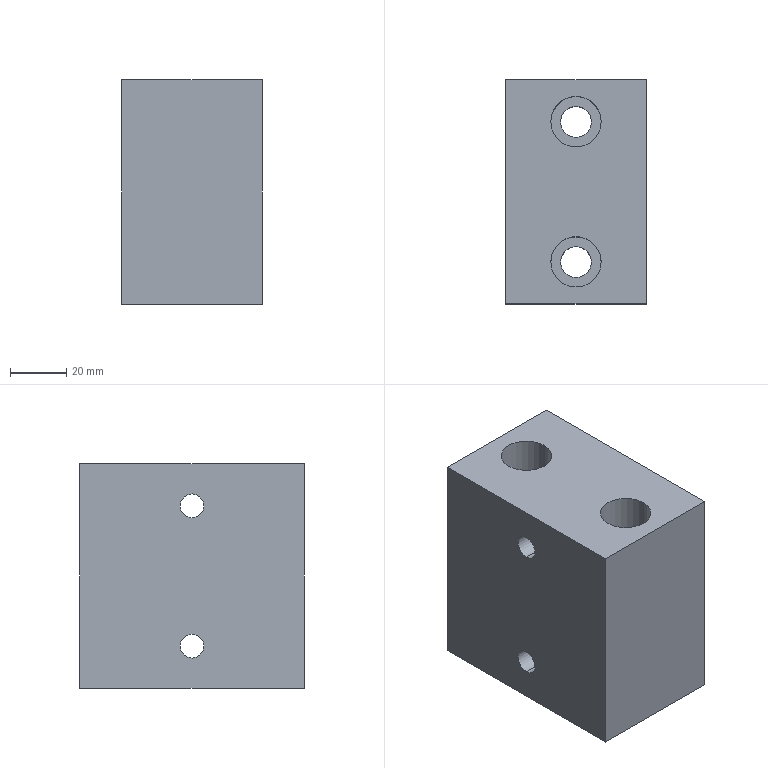Part | SolidWorks | features HoleWzd 2, Extrusion 1 | 1 solid | 20 faces | box 50 x 80 x 80 mm | volume 289554 mm3 | cylinder 12 | plane 8 | commonest cylinder face diameters 8.5 x4 11 x4 18 x4
STEP:
#1=CARTESIAN_POINT('',(0.,0.,-20.75));
#2=VERTEX_POINT('',#1);
#3=CARTESIAN_POINT('',(0.,0.,-29.25));
#4=VERTEX_POINT('',#3);
#5=CARTESIAN_POINT('',(0.,0.,-25.));
#6=DIRECTION('',(1.,0.,0.));
#7=DIRECTION('',(0.,0.,-1.));
#8=AXIS2_PLACEMENT_3D('',#5,#6,#7);
#9=CIRCLE('',#8,4.25);
#10=EDGE_CURVE('',#2,#4,#9,.T.);
#11=ORIENTED_EDGE('',*,*,#10,.F.);
#12=CARTESIAN_POINT('',(50.,0.,-20.75));
#13=VERTEX_POINT('',#12);
#14=CARTESIAN_POINT('',(50.,0.,-20.75));
#15=DIRECTION('',(1.,0.,0.));
#16=VECTOR('',#15,1000.);
#17=LINE('',#14,#16);
#18=EDGE_CURVE('',#2,#13,#17,.T.);
#19=ORIENTED_EDGE('',*,*,#18,.T.);
#20=CARTESIAN_POINT('',(50.,0.,-29.25));
#21=VERTEX_POINT('',#20);
#22=CARTESIAN_POINT('',(50.,0.,-25.));
#23=DIRECTION('',(1.,0.,0.));
#24=DIRECTION('',(0.,0.,-1.));
#25=AXIS2_PLACEMENT_3D('',#22,#23,#24);
#26=CIRCLE('',#25,4.25);
#27=EDGE_CURVE('',#13,#21,#26,.T.);
#28=ORIENTED_EDGE('',*,*,#27,.T.);
#29=CARTESIAN_POINT('',(50.,0.,-29.25));
#30=DIRECTION('',(1.,0.,0.));
#31=VECTOR('',#30,1000.);
#32=LINE('',#29,#31);
#33=EDGE_CURVE('',#4,#21,#32,.T.);
#34=ORIENTED_EDGE('',*,*,#33,.F.);
#35=EDGE_LOOP('',(#11,#19,#28,#34));
#36=FACE_OUTER_BOUND('',#35,.T.);
#37=CARTESIAN_POINT('',(50.,0.,-25.));
#38=DIRECTION('',(1.,0.,0.));
#39=DIRECTION('',(0.,0.,-1.));
#40=AXIS2_PLACEMENT_3D('',#37,#38,#39);
#41=CYLINDRICAL_SURFACE('',#40,4.25);
#42=ADVANCED_FACE('',(#36),#41,.F.);
#43=CARTESIAN_POINT('',(0.,0.,29.25));
#44=VERTEX_POINT('',#43);
#45=CARTESIAN_POINT('',(0.,0.,20.75));
#46=VERTEX_POINT('',#45);
#47=CARTESIAN_POINT('',(0.,0.,25.));
#48=DIRECTION('',(1.,0.,0.));
#49=DIRECTION('',(0.,0.,-1.));
#50=AXIS2_PLACEMENT_3D('',#47,#48,#49);
#51=CIRCLE('',#50,4.25);
#52=EDGE_CURVE('',#44,#46,#51,.T.);
#53=ORIENTED_EDGE('',*,*,#52,.F.);
#54=CARTESIAN_POINT('',(50.,0.,29.25));
#55=VERTEX_POINT('',#54);
#56=CARTESIAN_POINT('',(50.,0.,29.25));
#57=DIRECTION('',(1.,0.,0.));
#58=VECTOR('',#57,1000.);
#59=LINE('',#56,#58);
#60=EDGE_CURVE('',#44,#55,#59,.T.);
#61=ORIENTED_EDGE('',*,*,#60,.T.);
#62=CARTESIAN_POINT('',(50.,0.,20.75));
#63=VERTEX_POINT('',#62);
#64=CARTESIAN_POINT('',(50.,0.,25.));
#65=DIRECTION('',(1.,0.,0.));
#66=DIRECTION('',(0.,0.,-1.));
#67=AXIS2_PLACEMENT_3D('',#64,#65,#66);
#68=CIRCLE('',#67,4.25);
#69=EDGE_CURVE('',#55,#63,#68,.T.);
#70=ORIENTED_EDGE('',*,*,#69,.T.);
#71=CARTESIAN_POINT('',(50.,0.,20.75));
#72=DIRECTION('',(1.,0.,0.));
#73=VECTOR('',#72,1000.);
#74=LINE('',#71,#73);
#75=EDGE_CURVE('',#46,#63,#74,.T.);
#76=ORIENTED_EDGE('',*,*,#75,.F.);
#77=EDGE_LOOP('',(#53,#61,#70,#76));
#78=FACE_OUTER_BOUND('',#77,.T.);
#79=CARTESIAN_POINT('',(50.,0.,25.));
#80=DIRECTION('',(1.,0.,0.));
#81=DIRECTION('',(0.,0.,-1.));
#82=AXIS2_PLACEMENT_3D('',#79,#80,#81);
#83=CYLINDRICAL_SURFACE('',#82,4.25);
#84=ADVANCED_FACE('',(#78),#83,.F.);
#85=CARTESIAN_POINT('',(16.,25.,10.));
#86=VERTEX_POINT('',#85);
#87=CARTESIAN_POINT('',(34.,25.,10.));
#88=VERTEX_POINT('',#87);
#89=CARTESIAN_POINT('',(25.,25.,10.));
#90=DIRECTION('',(0.,0.,1.));
#91=DIRECTION('',(1.,0.,0.));
#92=AXIS2_PLACEMENT_3D('',#89,#90,#91);
#93=CIRCLE('',#92,9.);
#94=EDGE_CURVE('',#86,#88,#93,.T.);
#95=ORIENTED_EDGE('',*,*,#94,.F.);
#96=CARTESIAN_POINT('',(16.,25.,40.));
#97=VERTEX_POINT('',#96);
#98=CARTESIAN_POINT('',(16.,25.,40.));
#99=DIRECTION('',(0.,0.,1.));
#100=VECTOR('',#99,1000.);
#101=LINE('',#98,#100);
#102=EDGE_CURVE('',#86,#97,#101,.T.);
#103=ORIENTED_EDGE('',*,*,#102,.T.);
#104=CARTESIAN_POINT('',(34.,25.,40.));
#105=VERTEX_POINT('',#104);
#106=CARTESIAN_POINT('',(25.,25.,40.));
#107=DIRECTION('',(0.,0.,1.));
#108=DIRECTION('',(1.,0.,0.));
#109=AXIS2_PLACEMENT_3D('',#106,#107,#108);
#110=CIRCLE('',#109,9.);
#111=EDGE_CURVE('',#97,#105,#110,.T.);
#112=ORIENTED_EDGE('',*,*,#111,.T.);
#113=CARTESIAN_POINT('',(34.,25.,40.));
#114=DIRECTION('',(0.,0.,1.));
#115=VECTOR('',#114,1000.);
#116=LINE('',#113,#115);
#117=EDGE_CURVE('',#88,#105,#116,.T.);
#118=ORIENTED_EDGE('',*,*,#117,.F.);
#119=EDGE_LOOP('',(#95,#103,#112,#118));
#120=FACE_OUTER_BOUND('',#119,.T.);
#121=CARTESIAN_POINT('',(25.,25.,40.));
#122=DIRECTION('',(0.,0.,1.));
#123=DIRECTION('',(1.,0.,0.));
#124=AXIS2_PLACEMENT_3D('',#121,#122,#123);
#125=CYLINDRICAL_SURFACE('',#124,9.);
#126=ADVANCED_FACE('',(#120),#125,.F.);
#127=CARTESIAN_POINT('',(19.5,25.,-40.));
#128=VERTEX_POINT('',#127);
#129=CARTESIAN_POINT('',(30.5,25.,-40.));
#130=VERTEX_POINT('',#129);
#131=CARTESIAN_POINT('',(25.,25.,-40.));
#132=DIRECTION('',(0.,0.,1.));
#133=DIRECTION('',(1.,0.,0.));
#134=AXIS2_PLACEMENT_3D('',#131,#132,#133);
#135=CIRCLE('',#134,5.5);
#136=EDGE_CURVE('',#128,#130,#135,.T.);
#137=ORIENTED_EDGE('',*,*,#136,.F.);
#138=CARTESIAN_POINT('',(19.5,25.,10.));
#139=VERTEX_POINT('',#138);
#140=CARTESIAN_POINT('',(19.5,25.,40.));
#141=DIRECTION('',(0.,0.,1.));
#142=VECTOR('',#141,1000.);
#143=LINE('',#140,#142);
#144=EDGE_CURVE('',#128,#139,#143,.T.);
#145=ORIENTED_EDGE('',*,*,#144,.T.);
#146=CARTESIAN_POINT('',(30.5,25.,10.));
#147=VERTEX_POINT('',#146);
#148=CARTESIAN_POINT('',(25.,25.,10.));
#149=DIRECTION('',(0.,0.,1.));
#150=DIRECTION('',(1.,0.,0.));
#151=AXIS2_PLACEMENT_3D('',#148,#149,#150);
#152=CIRCLE('',#151,5.5);
#153=EDGE_CURVE('',#139,#147,#152,.T.);
#154=ORIENTED_EDGE('',*,*,#153,.T.);
#155=CARTESIAN_POINT('',(30.5,25.,40.));
#156=DIRECTION('',(0.,0.,1.));
#157=VECTOR('',#156,1000.);
#158=LINE('',#155,#157);
#159=EDGE_CURVE('',#130,#147,#158,.T.);
#160=ORIENTED_EDGE('',*,*,#159,.F.);
#161=EDGE_LOOP('',(#137,#145,#154,#160));
#162=FACE_OUTER_BOUND('',#161,.T.);
#163=CARTESIAN_POINT('',(25.,25.,40.));
#164=DIRECTION('',(0.,0.,1.));
#165=DIRECTION('',(1.,0.,0.));
#166=AXIS2_PLACEMENT_3D('',#163,#164,#165);
#167=CYLINDRICAL_SURFACE('',#166,5.5);
#168=ADVANCED_FACE('',(#162),#167,.F.);
#169=CARTESIAN_POINT('',(16.,-25.,10.));
#170=VERTEX_POINT('',#169);
#171=CARTESIAN_POINT('',(34.,-25.,10.));
#172=VERTEX_POINT('',#171);
#173=CARTESIAN_POINT('',(25.,-25.,10.));
#174=DIRECTION('',(0.,0.,1.));
#175=DIRECTION('',(1.,0.,0.));
#176=AXIS2_PLACEMENT_3D('',#173,#174,#175);
#177=CIRCLE('',#176,9.);
#178=EDGE_CURVE('',#170,#172,#177,.T.);
#179=ORIENTED_EDGE('',*,*,#178,.F.);
#180=CARTESIAN_POINT('',(16.,-25.,40.));
#181=VERTEX_POINT('',#180);
#182=CARTESIAN_POINT('',(16.,-25.,40.));
#183=DIRECTION('',(0.,0.,1.));
#184=VECTOR('',#183,1000.);
#185=LINE('',#182,#184);
#186=EDGE_CURVE('',#170,#181,#185,.T.);
#187=ORIENTED_EDGE('',*,*,#186,.T.);
#188=CARTESIAN_POINT('',(34.,-25.,40.));
#189=VERTEX_POINT('',#188);
#190=CARTESIAN_POINT('',(25.,-25.,40.));
#191=DIRECTION('',(0.,0.,1.));
#192=DIRECTION('',(1.,0.,0.));
#193=AXIS2_PLACEMENT_3D('',#190,#191,#192);
#194=CIRCLE('',#193,9.);
#195=EDGE_CURVE('',#181,#189,#194,.T.);
#196=ORIENTED_EDGE('',*,*,#195,.T.);
#197=CARTESIAN_POINT('',(34.,-25.,40.));
#198=DIRECTION('',(0.,0.,1.));
#199=VECTOR('',#198,1000.);
#200=LINE('',#197,#199);
#201=EDGE_CURVE('',#172,#189,#200,.T.);
#202=ORIENTED_EDGE('',*,*,#201,.F.);
#203=EDGE_LOOP('',(#179,#187,#196,#202));
#204=FACE_OUTER_BOUND('',#203,.T.);
#205=CARTESIAN_POINT('',(25.,-25.,40.));
#206=DIRECTION('',(0.,0.,1.));
#207=DIRECTION('',(1.,0.,0.));
#208=AXIS2_PLACEMENT_3D('',#205,#206,#207);
#209=CYLINDRICAL_SURFACE('',#208,9.);
#210=ADVANCED_FACE('',(#204),#209,.F.);
#211=CARTESIAN_POINT('',(19.5,-25.,-40.));
#212=VERTEX_POINT('',#211);
#213=CARTESIAN_POINT('',(30.5,-25.,-40.));
#214=VERTEX_POINT('',#213);
#215=CARTESIAN_POINT('',(25.,-25.,-40.));
#216=DIRECTION('',(0.,0.,1.));
#217=DIRECTION('',(1.,0.,0.));
#218=AXIS2_PLACEMENT_3D('',#215,#216,#217);
#219=CIRCLE('',#218,5.5);
#220=EDGE_CURVE('',#212,#214,#219,.T.);
#221=ORIENTED_EDGE('',*,*,#220,.F.);
#222=CARTESIAN_POINT('',(19.5,-25.,10.));
#223=VERTEX_POINT('',#222);
#224=CARTESIAN_POINT('',(19.5,-25.,40.));
#225=DIRECTION('',(0.,0.,1.));
#226=VECTOR('',#225,1000.);
#227=LINE('',#224,#226);
#228=EDGE_CURVE('',#212,#223,#227,.T.);
#229=ORIENTED_EDGE('',*,*,#228,.T.);
#230=CARTESIAN_POINT('',(30.5,-25.,10.));
#231=VERTEX_POINT('',#230);
#232=CARTESIAN_POINT('',(25.,-25.,10.));
#233=DIRECTION('',(0.,0.,1.));
#234=DIRECTION('',(1.,0.,0.));
#235=AXIS2_PLACEMENT_3D('',#232,#233,#234);
#236=CIRCLE('',#235,5.5);
#237=EDGE_CURVE('',#223,#231,#236,.T.);
#238=ORIENTED_EDGE('',*,*,#237,.T.);
#239=CARTESIAN_POINT('',(30.5,-25.,40.));
#240=DIRECTION('',(0.,0.,1.));
#241=VECTOR('',#240,1000.);
#242=LINE('',#239,#241);
#243=EDGE_CURVE('',#214,#231,#242,.T.);
#244=ORIENTED_EDGE('',*,*,#243,.F.);
#245=EDGE_LOOP('',(#221,#229,#238,#244));
#246=FACE_OUTER_BOUND('',#245,.T.);
#247=CARTESIAN_POINT('',(25.,-25.,40.));
#248=DIRECTION('',(0.,0.,1.));
#249=DIRECTION('',(1.,0.,0.));
#250=AXIS2_PLACEMENT_3D('',#247,#248,#249);
#251=CYLINDRICAL_SURFACE('',#250,5.5);
#252=ADVANCED_FACE('',(#246),#251,.F.);
#253=CARTESIAN_POINT('',(25.,25.,-40.));
#254=DIRECTION('',(0.,0.,1.));
#255=DIRECTION('',(1.,0.,0.));
#256=AXIS2_PLACEMENT_3D('',#253,#254,#255);
#257=CIRCLE('',#256,5.5);
#258=EDGE_CURVE('',#130,#128,#257,.T.);
#259=ORIENTED_EDGE('',*,*,#258,.T.);
#260=ORIENTED_EDGE('',*,*,#136,.T.);
#261=EDGE_LOOP('',(#259,#260));
#262=FACE_BOUND('',#261,.T.);
#263=CARTESIAN_POINT('',(25.,-25.,-40.));
#264=DIRECTION('',(0.,0.,1.));
#265=DIRECTION('',(1.,0.,0.));
#266=AXIS2_PLACEMENT_3D('',#263,#264,#265);
#267=CIRCLE('',#266,5.5);
#268=EDGE_CURVE('',#214,#212,#267,.T.);
#269=ORIENTED_EDGE('',*,*,#268,.T.);
#270=ORIENTED_EDGE('',*,*,#220,.T.);
#271=EDGE_LOOP('',(#269,#270));
#272=FACE_BOUND('',#271,.T.);
#273=CARTESIAN_POINT('',(0.,-40.,-40.));
#274=VERTEX_POINT('',#273);
#275=CARTESIAN_POINT('',(0.,40.,-40.));
#276=VERTEX_POINT('',#275);
#277=CARTESIAN_POINT('',(0.,40.,-40.));
#278=DIRECTION('',(0.,1.,0.));
#279=VECTOR('',#278,1000.);
#280=LINE('',#277,#279);
#281=EDGE_CURVE('',#274,#276,#280,.T.);
#282=ORIENTED_EDGE('',*,*,#281,.T.);
#283=CARTESIAN_POINT('',(50.,40.,-40.));
#284=VERTEX_POINT('',#283);
#285=CARTESIAN_POINT('',(50.,40.,-40.));
#286=DIRECTION('',(-1.,0.,0.));
#287=VECTOR('',#286,1000.);
#288=LINE('',#285,#287);
#289=EDGE_CURVE('',#284,#276,#288,.T.);
#290=ORIENTED_EDGE('',*,*,#289,.F.);
#291=CARTESIAN_POINT('',(50.,-40.,-40.));
#292=VERTEX_POINT('',#291);
#293=CARTESIAN_POINT('',(50.,40.,-40.));
#294=DIRECTION('',(0.,1.,0.));
#295=VECTOR('',#294,1000.);
#296=LINE('',#293,#295);
#297=EDGE_CURVE('',#292,#284,#296,.T.);
#298=ORIENTED_EDGE('',*,*,#297,.F.);
#299=CARTESIAN_POINT('',(50.,-40.,-40.));
#300=DIRECTION('',(-1.,0.,0.));
#301=VECTOR('',#300,1000.);
#302=LINE('',#299,#301);
#303=EDGE_CURVE('',#292,#274,#302,.T.);
#304=ORIENTED_EDGE('',*,*,#303,.T.);
#305=EDGE_LOOP('',(#282,#290,#298,#304));
#306=FACE_OUTER_BOUND('',#305,.T.);
#307=CARTESIAN_POINT('',(50.,40.,-40.));
#308=DIRECTION('',(0.,0.,1.));
#309=DIRECTION('',(0.,-1.,0.));
#310=AXIS2_PLACEMENT_3D('',#307,#308,#309);
#311=PLANE('',#310);
#312=ADVANCED_FACE('',(#262,#272,#306),#311,.F.);
#313=CARTESIAN_POINT('',(0.,40.,40.));
#314=VERTEX_POINT('',#313);
#315=CARTESIAN_POINT('',(0.,40.,40.));
#316=DIRECTION('',(0.,0.,1.));
#317=VECTOR('',#316,1000.);
#318=LINE('',#315,#317);
#319=EDGE_CURVE('',#276,#314,#318,.T.);
#320=ORIENTED_EDGE('',*,*,#319,.T.);
#321=CARTESIAN_POINT('',(50.,40.,40.));
#322=VERTEX_POINT('',#321);
#323=CARTESIAN_POINT('',(50.,40.,40.));
#324=DIRECTION('',(-1.,0.,0.));
#325=VECTOR('',#324,1000.);
#326=LINE('',#323,#325);
#327=EDGE_CURVE('',#322,#314,#326,.T.);
#328=ORIENTED_EDGE('',*,*,#327,.F.);
#329=CARTESIAN_POINT('',(50.,40.,40.));
#330=DIRECTION('',(0.,0.,1.));
#331=VECTOR('',#330,1000.);
#332=LINE('',#329,#331);
#333=EDGE_CURVE('',#284,#322,#332,.T.);
#334=ORIENTED_EDGE('',*,*,#333,.F.);
#335=ORIENTED_EDGE('',*,*,#289,.T.);
#336=EDGE_LOOP('',(#320,#328,#334,#335));
#337=FACE_OUTER_BOUND('',#336,.T.);
#338=CARTESIAN_POINT('',(50.,40.,40.));
#339=DIRECTION('',(0.,-1.,0.));
#340=DIRECTION('',(0.,0.,-1.));
#341=AXIS2_PLACEMENT_3D('',#338,#339,#340);
#342=PLANE('',#341);
#343=ADVANCED_FACE('',(#337),#342,.F.);
#344=CARTESIAN_POINT('',(25.,25.,40.));
#345=DIRECTION('',(0.,0.,1.));
#346=DIRECTION('',(1.,0.,0.));
#347=AXIS2_PLACEMENT_3D('',#344,#345,#346);
#348=CIRCLE('',#347,9.);
#349=EDGE_CURVE('',#105,#97,#348,.T.);
#350=ORIENTED_EDGE('',*,*,#349,.F.);
#351=ORIENTED_EDGE('',*,*,#111,.F.);
#352=EDGE_LOOP('',(#350,#351));
#353=FACE_BOUND('',#352,.T.);
#354=CARTESIAN_POINT('',(25.,-25.,40.));
#355=DIRECTION('',(0.,0.,1.));
#356=DIRECTION('',(1.,0.,0.));
#357=AXIS2_PLACEMENT_3D('',#354,#355,#356);
#358=CIRCLE('',#357,9.);
#359=EDGE_CURVE('',#189,#181,#358,.T.);
#360=ORIENTED_EDGE('',*,*,#359,.F.);
#361=ORIENTED_EDGE('',*,*,#195,.F.);
#362=EDGE_LOOP('',(#360,#361));
#363=FACE_BOUND('',#362,.T.);
#364=CARTESIAN_POINT('',(0.,-40.,40.));
#365=VERTEX_POINT('',#364);
#366=CARTESIAN_POINT('',(0.,40.,40.));
#367=DIRECTION('',(0.,-1.,0.));
#368=VECTOR('',#367,1000.);
#369=LINE('',#366,#368);
#370=EDGE_CURVE('',#314,#365,#369,.T.);
#371=ORIENTED_EDGE('',*,*,#370,.T.);
#372=CARTESIAN_POINT('',(50.,-40.,40.));
#373=VERTEX_POINT('',#372);
#374=CARTESIAN_POINT('',(50.,-40.,40.));
#375=DIRECTION('',(-1.,0.,0.));
#376=VECTOR('',#375,1000.);
#377=LINE('',#374,#376);
#378=EDGE_CURVE('',#373,#365,#377,.T.);
#379=ORIENTED_EDGE('',*,*,#378,.F.);
#380=CARTESIAN_POINT('',(50.,40.,40.));
#381=DIRECTION('',(0.,-1.,0.));
#382=VECTOR('',#381,1000.);
#383=LINE('',#380,#382);
#384=EDGE_CURVE('',#322,#373,#383,.T.);
#385=ORIENTED_EDGE('',*,*,#384,.F.);
#386=ORIENTED_EDGE('',*,*,#327,.T.);
#387=EDGE_LOOP('',(#371,#379,#385,#386));
#388=FACE_OUTER_BOUND('',#387,.T.);
#389=CARTESIAN_POINT('',(50.,40.,40.));
#390=DIRECTION('',(0.,0.,-1.));
#391=DIRECTION('',(0.,1.,0.));
#392=AXIS2_PLACEMENT_3D('',#389,#390,#391);
#393=PLANE('',#392);
#394=ADVANCED_FACE('',(#353,#363,#388),#393,.F.);
#395=CARTESIAN_POINT('',(0.,-40.,40.));
#396=DIRECTION('',(0.,0.,-1.));
#397=VECTOR('',#396,1000.);
#398=LINE('',#395,#397);
#399=EDGE_CURVE('',#365,#274,#398,.T.);
#400=ORIENTED_EDGE('',*,*,#399,.T.);
#401=ORIENTED_EDGE('',*,*,#303,.F.);
#402=CARTESIAN_POINT('',(50.,-40.,40.));
#403=DIRECTION('',(0.,0.,-1.));
#404=VECTOR('',#403,1000.);
#405=LINE('',#402,#404);
#406=EDGE_CURVE('',#373,#292,#405,.T.);
#407=ORIENTED_EDGE('',*,*,#406,.F.);
#408=ORIENTED_EDGE('',*,*,#378,.T.);
#409=EDGE_LOOP('',(#400,#401,#407,#408));
#410=FACE_OUTER_BOUND('',#409,.T.);
#411=CARTESIAN_POINT('',(50.,-40.,40.));
#412=DIRECTION('',(0.,1.,0.));
#413=DIRECTION('',(0.,0.,1.));
#414=AXIS2_PLACEMENT_3D('',#411,#412,#413);
#415=PLANE('',#414);
#416=ADVANCED_FACE('',(#410),#415,.F.);
#417=CARTESIAN_POINT('',(50.,0.,-25.));
#418=DIRECTION('',(1.,0.,0.));
#419=DIRECTION('',(0.,0.,-1.));
#420=AXIS2_PLACEMENT_3D('',#417,#418,#419);
#421=CIRCLE('',#420,4.25);
#422=EDGE_CURVE('',#21,#13,#421,.T.);
#423=ORIENTED_EDGE('',*,*,#422,.F.);
#424=ORIENTED_EDGE('',*,*,#27,.F.);
#425=EDGE_LOOP('',(#423,#424));
#426=FACE_BOUND('',#425,.T.);
#427=CARTESIAN_POINT('',(50.,0.,25.));
#428=DIRECTION('',(1.,0.,0.));
#429=DIRECTION('',(0.,0.,-1.));
#430=AXIS2_PLACEMENT_3D('',#427,#428,#429);
#431=CIRCLE('',#430,4.25);
#432=EDGE_CURVE('',#63,#55,#431,.T.);
#433=ORIENTED_EDGE('',*,*,#432,.F.);
#434=ORIENTED_EDGE('',*,*,#69,.F.);
#435=EDGE_LOOP('',(#433,#434));
#436=FACE_BOUND('',#435,.T.);
#437=ORIENTED_EDGE('',*,*,#297,.T.);
#438=ORIENTED_EDGE('',*,*,#333,.T.);
#439=ORIENTED_EDGE('',*,*,#384,.T.);
#440=ORIENTED_EDGE('',*,*,#406,.T.);
#441=EDGE_LOOP('',(#437,#438,#439,#440));
#442=FACE_OUTER_BOUND('',#441,.T.);
#443=CARTESIAN_POINT('',(50.,0.,0.));
#444=DIRECTION('',(1.,0.,0.));
#445=DIRECTION('',(0.,0.,-1.));
#446=AXIS2_PLACEMENT_3D('',#443,#444,#445);
#447=PLANE('',#446);
#448=ADVANCED_FACE('',(#426,#436,#442),#447,.T.);
#449=CARTESIAN_POINT('',(0.,0.,-25.));
#450=DIRECTION('',(1.,0.,0.));
#451=DIRECTION('',(0.,0.,-1.));
#452=AXIS2_PLACEMENT_3D('',#449,#450,#451);
#453=CIRCLE('',#452,4.25);
#454=EDGE_CURVE('',#4,#2,#453,.T.);
#455=ORIENTED_EDGE('',*,*,#454,.T.);
#456=ORIENTED_EDGE('',*,*,#10,.T.);
#457=EDGE_LOOP('',(#455,#456));
#458=FACE_BOUND('',#457,.T.);
#459=CARTESIAN_POINT('',(0.,0.,25.));
#460=DIRECTION('',(1.,0.,0.));
#461=DIRECTION('',(0.,0.,-1.));
#462=AXIS2_PLACEMENT_3D('',#459,#460,#461);
#463=CIRCLE('',#462,4.25);
#464=EDGE_CURVE('',#46,#44,#463,.T.);
#465=ORIENTED_EDGE('',*,*,#464,.T.);
#466=ORIENTED_EDGE('',*,*,#52,.T.);
#467=EDGE_LOOP('',(#465,#466));
#468=FACE_BOUND('',#467,.T.);
#469=ORIENTED_EDGE('',*,*,#281,.F.);
#470=ORIENTED_EDGE('',*,*,#399,.F.);
#471=ORIENTED_EDGE('',*,*,#370,.F.);
#472=ORIENTED_EDGE('',*,*,#319,.F.);
#473=EDGE_LOOP('',(#469,#470,#471,#472));
#474=FACE_OUTER_BOUND('',#473,.T.);
#475=CARTESIAN_POINT('',(0.,0.,0.));
#476=DIRECTION('',(1.,0.,0.));
#477=DIRECTION('',(0.,0.,-1.));
#478=AXIS2_PLACEMENT_3D('',#475,#476,#477);
#479=PLANE('',#478);
#480=ADVANCED_FACE('',(#458,#468,#474),#479,.F.);
#481=ORIENTED_EDGE('',*,*,#228,.F.);
#482=ORIENTED_EDGE('',*,*,#268,.F.);
#483=ORIENTED_EDGE('',*,*,#243,.T.);
#484=CARTESIAN_POINT('',(25.,-25.,10.));
#485=DIRECTION('',(0.,0.,1.));
#486=DIRECTION('',(1.,0.,0.));
#487=AXIS2_PLACEMENT_3D('',#484,#485,#486);
#488=CIRCLE('',#487,5.5);
#489=EDGE_CURVE('',#231,#223,#488,.T.);
#490=ORIENTED_EDGE('',*,*,#489,.T.);
#491=EDGE_LOOP('',(#481,#482,#483,#490));
#492=FACE_OUTER_BOUND('',#491,.T.);
#493=CARTESIAN_POINT('',(25.,-25.,40.));
#494=DIRECTION('',(0.,0.,1.));
#495=DIRECTION('',(1.,0.,0.));
#496=AXIS2_PLACEMENT_3D('',#493,#494,#495);
#497=CYLINDRICAL_SURFACE('',#496,5.5);
#498=ADVANCED_FACE('',(#492),#497,.F.);
#499=ORIENTED_EDGE('',*,*,#489,.F.);
#500=ORIENTED_EDGE('',*,*,#237,.F.);
#501=EDGE_LOOP('',(#499,#500));
#502=FACE_BOUND('',#501,.T.);
#503=CARTESIAN_POINT('',(25.,-25.,10.));
#504=DIRECTION('',(0.,0.,1.));
#505=DIRECTION('',(1.,0.,0.));
#506=AXIS2_PLACEMENT_3D('',#503,#504,#505);
#507=CIRCLE('',#506,9.);
#508=EDGE_CURVE('',#172,#170,#507,.T.);
#509=ORIENTED_EDGE('',*,*,#508,.T.);
#510=ORIENTED_EDGE('',*,*,#178,.T.);
#511=EDGE_LOOP('',(#509,#510));
#512=FACE_OUTER_BOUND('',#511,.T.);
#513=CARTESIAN_POINT('',(30.5,-25.,10.));
#514=DIRECTION('',(0.,0.,-1.));
#515=DIRECTION('',(-1.,0.,0.));
#516=AXIS2_PLACEMENT_3D('',#513,#514,#515);
#517=PLANE('',#516);
#518=ADVANCED_FACE('',(#502,#512),#517,.F.);
#519=ORIENTED_EDGE('',*,*,#186,.F.);
#520=ORIENTED_EDGE('',*,*,#508,.F.);
#521=ORIENTED_EDGE('',*,*,#201,.T.);
#522=ORIENTED_EDGE('',*,*,#359,.T.);
#523=EDGE_LOOP('',(#519,#520,#521,#522));
#524=FACE_OUTER_BOUND('',#523,.T.);
#525=CARTESIAN_POINT('',(25.,-25.,40.));
#526=DIRECTION('',(0.,0.,1.));
#527=DIRECTION('',(1.,0.,0.));
#528=AXIS2_PLACEMENT_3D('',#525,#526,#527);
#529=CYLINDRICAL_SURFACE('',#528,9.);
#530=ADVANCED_FACE('',(#524),#529,.F.);
#531=ORIENTED_EDGE('',*,*,#144,.F.);
#532=ORIENTED_EDGE('',*,*,#258,.F.);
#533=ORIENTED_EDGE('',*,*,#159,.T.);
#534=CARTESIAN_POINT('',(25.,25.,10.));
#535=DIRECTION('',(0.,0.,1.));
#536=DIRECTION('',(1.,0.,0.));
#537=AXIS2_PLACEMENT_3D('',#534,#535,#536);
#538=CIRCLE('',#537,5.5);
#539=EDGE_CURVE('',#147,#139,#538,.T.);
#540=ORIENTED_EDGE('',*,*,#539,.T.);
#541=EDGE_LOOP('',(#531,#532,#533,#540));
#542=FACE_OUTER_BOUND('',#541,.T.);
#543=CARTESIAN_POINT('',(25.,25.,40.));
#544=DIRECTION('',(0.,0.,1.));
#545=DIRECTION('',(1.,0.,0.));
#546=AXIS2_PLACEMENT_3D('',#543,#544,#545);
#547=CYLINDRICAL_SURFACE('',#546,5.5);
#548=ADVANCED_FACE('',(#542),#547,.F.);
#549=ORIENTED_EDGE('',*,*,#539,.F.);
#550=ORIENTED_EDGE('',*,*,#153,.F.);
#551=EDGE_LOOP('',(#549,#550));
#552=FACE_BOUND('',#551,.T.);
#553=CARTESIAN_POINT('',(25.,25.,10.));
#554=DIRECTION('',(0.,0.,1.));
#555=DIRECTION('',(1.,0.,0.));
#556=AXIS2_PLACEMENT_3D('',#553,#554,#555);
#557=CIRCLE('',#556,9.);
#558=EDGE_CURVE('',#88,#86,#557,.T.);
#559=ORIENTED_EDGE('',*,*,#558,.T.);
#560=ORIENTED_EDGE('',*,*,#94,.T.);
#561=EDGE_LOOP('',(#559,#560));
#562=FACE_OUTER_BOUND('',#561,.T.);
#563=CARTESIAN_POINT('',(30.5,25.,10.));
#564=DIRECTION('',(0.,0.,-1.));
#565=DIRECTION('',(-1.,0.,0.));
#566=AXIS2_PLACEMENT_3D('',#563,#564,#565);
#567=PLANE('',#566);
#568=ADVANCED_FACE('',(#552,#562),#567,.F.);
#569=ORIENTED_EDGE('',*,*,#102,.F.);
#570=ORIENTED_EDGE('',*,*,#558,.F.);
#571=ORIENTED_EDGE('',*,*,#117,.T.);
#572=ORIENTED_EDGE('',*,*,#349,.T.);
#573=EDGE_LOOP('',(#569,#570,#571,#572));
#574=FACE_OUTER_BOUND('',#573,.T.);
#575=CARTESIAN_POINT('',(25.,25.,40.));
#576=DIRECTION('',(0.,0.,1.));
#577=DIRECTION('',(1.,0.,0.));
#578=AXIS2_PLACEMENT_3D('',#575,#576,#577);
#579=CYLINDRICAL_SURFACE('',#578,9.);
#580=ADVANCED_FACE('',(#574),#579,.F.);
#581=ORIENTED_EDGE('',*,*,#60,.F.);
#582=ORIENTED_EDGE('',*,*,#464,.F.);
#583=ORIENTED_EDGE('',*,*,#75,.T.);
#584=ORIENTED_EDGE('',*,*,#432,.T.);
#585=EDGE_LOOP('',(#581,#582,#583,#584));
#586=FACE_OUTER_BOUND('',#585,.T.);
#587=CARTESIAN_POINT('',(50.,0.,25.));
#588=DIRECTION('',(1.,0.,0.));
#589=DIRECTION('',(0.,0.,-1.));
#590=AXIS2_PLACEMENT_3D('',#587,#588,#589);
#591=CYLINDRICAL_SURFACE('',#590,4.25);
#592=ADVANCED_FACE('',(#586),#591,.F.);
#593=ORIENTED_EDGE('',*,*,#18,.F.);
#594=ORIENTED_EDGE('',*,*,#454,.F.);
#595=ORIENTED_EDGE('',*,*,#33,.T.);
#596=ORIENTED_EDGE('',*,*,#422,.T.);
#597=EDGE_LOOP('',(#593,#594,#595,#596));
#598=FACE_OUTER_BOUND('',#597,.T.);
#599=CARTESIAN_POINT('',(50.,0.,-25.));
#600=DIRECTION('',(1.,0.,0.));
#601=DIRECTION('',(0.,0.,-1.));
#602=AXIS2_PLACEMENT_3D('',#599,#600,#601);
#603=CYLINDRICAL_SURFACE('',#602,4.25);
#604=ADVANCED_FACE('',(#598),#603,.F.);
#605=CLOSED_SHELL('',(#42,#84,#126,#168,#210,#252,#312,#343,#394,#416,#448,#480,#498,#518,#530,#548,#568,#580,#592,#604));
#606=MANIFOLD_SOLID_BREP('',#605);
#607=CARTESIAN_POINT('',(0.,0.,0.));
#608=DIRECTION('',(0.,0.,1.));
#609=DIRECTION('',(1.,0.,0.));
#610=AXIS2_PLACEMENT_3D('',#607,#608,#609);
#611=(LENGTH_UNIT()NAMED_UNIT(*)SI_UNIT(.MILLI.,.METRE.));
#612=UNCERTAINTY_MEASURE_WITH_UNIT(LENGTH_MEASURE(0.00001),#611,'','');
#613=(NAMED_UNIT(*)PLANE_ANGLE_UNIT()SI_UNIT($,.RADIAN.));
#614=(NAMED_UNIT(*)SI_UNIT($,.STERADIAN.)SOLID_ANGLE_UNIT());
#615=(GEOMETRIC_REPRESENTATION_CONTEXT(3)GLOBAL_UNCERTAINTY_ASSIGNED_CONTEXT((#612))GLOBAL_UNIT_ASSIGNED_CONTEXT((#611,#613,#614))REPRESENTATION_CONTEXT('',''));
#616=ADVANCED_BREP_SHAPE_REPRESENTATION('',(#606,#610),#615);